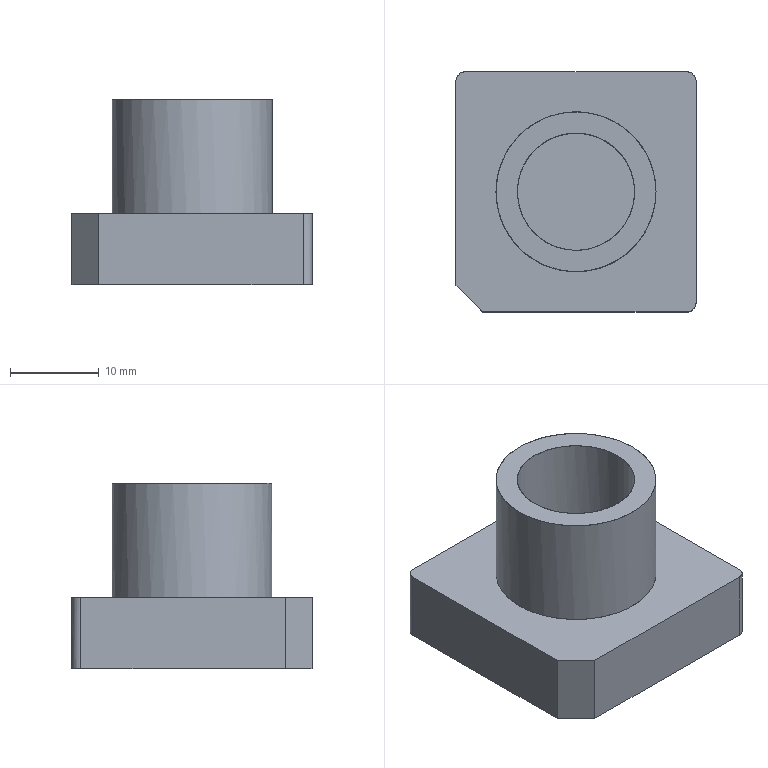NC program | PowerMill | posted with a generic post | part box 27 x 27 x 20.913 mm
Lines 1 to 1038 of 92133:
%
O0001
N104 ( POWERMILL CB  : 2026004.0)
N105 ( POST VER      : 2026.0.0.5161)
N106 ( OPTION FILE   : FANUC)
N107 ( OUTPUT WORKPLANE : WORLD)
N108 (  )
N109 ( TOOL LIST )
N110 (---------------------------------------)
N111 ( NO. | ID        | DIA.| TIP RAD|LENGTH)
N112 (---------------------------------------)
N113 (    1|D10C_1_1_1 |10.0 |  0.0   |76.36 )
N114 (    2|D4C_1_1    | 4.0 |  0.0   |68.12 )
N115 (    3|D10_1_1_1  |10.0 |  0.0   |76.08 )
N116 (   14|D4_1_1     | 4.0 |  0.0   |66.84 )
N117 (   13|TEXT_D4_1_1| 4.0 |  0.3   |68.16 )
N118 (---------------------------------------)
N119 (  )
N120 ( NUMBER OF TOOLPATHS: 11.0 )
N121 ( ESTIMATED PROGRAM DURATION: 0 HOURS 9 MIN 20 SEC)
N122 (  )
N123 G00 G21 G80 G40 G17
N124 G90
N125 G54
N126 G53 Z0.0
N127 (---------------)
N128 ( START TOOLPATH : 精公开粗01-扫面平行-D10C )
N129 (---------------)
N130 ( TOOL NO.    :1 )
N131 ( TOOL TYPE   : ENDMILL)
N132 ( TOOL ID     : D10C_1_1_1)
N133 ( TOOL DIA    : 10.0 LENGTH 76.36)
N134 T1
N135 M6
N136 S8000 M03
N137 G00 G90 X0.0 Y0.0
N138 G43 Z10.2 H1
N139
N140 G05 P10000 R4
N141 X21.28 Y16.28
N142 Z1.133
N143 G01 Z-0.067 F6000.0
N144 X16.28 F10000.0
N145 X-16.28
N146 Y10.8533
N147 X16.28
N148 Y5.4267
N149 X-16.28
N150 Y0.0
N151 X16.28
N152 Y-5.4267
N153 X-16.28
N154 Y-10.8533
N155 X16.28
N156 Y-16.28
N157 X-16.28
N158 X-21.28
N159 G00 Z10.2
N160 G05 P0
N161 (---------------)
N162 ( END TOOLPATH : 精公开粗01-扫面平行-D10C )
N163 (---------------)
N164 ( START TOOLPATH : 精公开粗01-外形偏置-D10C )
N165 (---------------)
N166 G00 X0.0 Y0.0 Z9.883
N167 G05 P10000 R4
N168 X22.054 Y5.4447
N169 Z0.6836
N170 G01 Z-0.5164 F6000.0
N171 X21.5265 F10000.0
N172 G03 X16.779 Y0.6972 I0.0 J-4.7475
N173 G01 Y-15.779
N174 G02 X15.779 Y-16.779 I-1.0 J0.0
N175 G01 X-15.779
N176 G02 X-16.779 Y-15.779 I0.0 J1.0
N177 G01 Y15.779
N178 G02 X-15.779 Y16.779 I1.0 J0.0
N179 G01 X15.779
N180 G02 X16.779 Y15.779 I0.0 J-1.0
N181 G01 Y0.6972
N182 X14.2597 Y0.5801
N183 X14.2687 Y0.3867
N184 Y-0.3867
N185 X14.2328 Y-1.1601
N186 X14.1427 Y-1.9336
N187 X14.0142 Y-2.707
N188 X13.8493 Y-3.4804
N189 X13.535 Y-4.5492
N190 X13.0486 Y-5.8007
N191 X12.7615 Y-6.4061
N192 X12.2358 Y-7.3476
N193 X11.7458 Y-8.121
N194 X11.1691 Y-8.8944
N195 X10.4413 Y-9.7288
N196 X9.7338 Y-10.4413
N197 X8.838 Y-11.2147
N198 X8.121 Y-11.7458
N199 X7.3476 Y-12.2446
N200 X6.5741 Y-12.6678
N201 X5.8007 Y-13.0486
N202 X4.5493 Y-13.535
N203 X3.4804 Y-13.8493
N204 X2.707 Y-14.02
N205 X1.9336 Y-14.1424
N206 X1.1601 Y-14.2328
N207 X-0.3867 Y-14.2747
N208 X-1.1601 Y-14.2328
N209 X-1.9336 Y-14.1478
N210 X-2.707 Y-14.0142
N211 X-3.4804 Y-13.8493
N212 X-4.5492 Y-13.535
N213 X-5.8007 Y-13.0486
N214 X-6.5741 Y-12.676
N215 X-7.3476 Y-12.2358
N216 X-8.121 Y-11.7458
N217 X-8.8944 Y-11.1654
N218 X-9.7288 Y-10.4413
N219 X-10.4413 Y-9.7404
N220 X-11.1654 Y-8.8944
N221 X-11.7458 Y-8.121
N222 X-11.9881 Y-7.7458
N223 X-12.6678 Y-6.5741
N224 X-13.0486 Y-5.8007
N225 X-13.535 Y-4.5492
N226 X-13.8493 Y-3.4804
N227 X-14.0164 Y-2.707
N228 X-14.1424 Y-1.9336
N229 X-14.2328 Y-1.1601
N230 X-14.2687 Y-0.3867
N231 Y0.3867
N232 X-14.2328 Y1.1601
N233 X-14.1424 Y1.9336
N234 X-14.0164 Y2.707
N235 X-13.8493 Y3.4804
N236 X-13.535 Y4.5493
N237 X-13.0486 Y5.8007
N238 X-12.6678 Y6.5741
N239 X-12.2358 Y7.3476
N240 X-11.7458 Y8.121
N241 X-11.1654 Y8.8944
N242 X-10.5096 Y9.6678
N243 X-9.7288 Y10.4413
N244 X-8.8944 Y11.1654
N245 X-8.121 Y11.7458
N246 X-7.7458 Y11.9881
N247 X-6.5741 Y12.676
N248 X-5.8007 Y13.0486
N249 X-4.5492 Y13.535
N250 X-3.4804 Y13.8493
N251 X-2.707 Y14.0142
N252 X-1.9336 Y14.1478
N253 X-1.1601 Y14.2328
N254 X-0.3867 Y14.2747
N255 X1.1601 Y14.2328
N256 X1.9336 Y14.1424
N257 X2.707 Y14.02
N258 X3.4804 Y13.8493
N259 X4.5493 Y13.535
N260 X5.8007 Y13.0486
N261 X6.5741 Y12.6678
N262 X7.3476 Y12.2446
N263 X8.121 Y11.7458
N264 X8.838 Y11.2147
N265 X9.7338 Y10.4413
N266 X10.4413 Y9.7288
N267 X11.1691 Y8.8944
N268 X11.7458 Y8.121
N269 X11.9881 Y7.7588
N270 X12.7615 Y6.4061
N271 X13.0486 Y5.8007
N272 X13.535 Y4.5493
N273 X13.8493 Y3.4804
N274 X14.0142 Y2.707
N275 X14.1427 Y1.9336
N276 X14.2328 Y1.1601
N277 X14.2597 Y0.5801
N278 X16.779 Y0.6972
N279 G00 Z3.2842
N280 G01 X22.054 Y5.4447
N281 G00 Z0.2842
N282 G01 Z-0.9158 F6000.0
N283 X21.5265 F10000.0
N284 G03 X16.779 Y0.6972 I0.0 J-4.7475
N285 G01 Y-15.779
N286 G02 X15.779 Y-16.779 I-1.0 J0.0
N287 G01 X-15.779
N288 G02 X-16.779 Y-15.779 I0.0 J1.0
N289 G01 Y15.779
N290 G02 X-15.779 Y16.779 I1.0 J0.0
N291 G01 X15.779
N292 G02 X16.779 Y15.779 I0.0 J-1.0
N293 G01 Y0.6972
N294 X14.2597 Y0.5801
N295 X14.2687 Y0.3867
N296 Y-0.3867
N297 X14.2328 Y-1.1601
N298 X14.1427 Y-1.9336
N299 X14.0142 Y-2.707
N300 X13.8493 Y-3.4804
N301 X13.535 Y-4.5492
N302 X13.0486 Y-5.8007
N303 X12.7615 Y-6.4061
N304 X12.2358 Y-7.3476
N305 X11.7458 Y-8.121
N306 X11.1691 Y-8.8944
N307 X10.4413 Y-9.7288
N308 X9.7338 Y-10.4413
N309 X8.838 Y-11.2147
N310 X8.121 Y-11.7458
N311 X7.3476 Y-12.2446
N312 X6.5741 Y-12.6678
N313 X5.8007 Y-13.0486
N314 X4.5493 Y-13.535
N315 X3.4804 Y-13.8493
N316 X2.707 Y-14.02
N317 X1.9336 Y-14.1424
N318 X1.1601 Y-14.2328
N319 X-0.3867 Y-14.2747
N320 X-1.1601 Y-14.2328
N321 X-1.9336 Y-14.1478
N322 X-2.707 Y-14.0142
N323 X-3.4804 Y-13.8493
N324 X-4.5492 Y-13.535
N325 X-5.8007 Y-13.0486
N326 X-6.5741 Y-12.676
N327 X-7.3476 Y-12.2358
N328 X-8.121 Y-11.7458
N329 X-8.8944 Y-11.1654
N330 X-9.7288 Y-10.4413
N331 X-10.4413 Y-9.7404
N332 X-11.1654 Y-8.8944
N333 X-11.7458 Y-8.121
N334 X-11.9881 Y-7.7459
N335 X-12.6678 Y-6.5741
N336 X-13.0486 Y-5.8007
N337 X-13.535 Y-4.5492
N338 X-13.8493 Y-3.4804
N339 X-14.0164 Y-2.707
N340 X-14.1424 Y-1.9336
N341 X-14.2328 Y-1.1601
N342 X-14.2687 Y-0.3867
N343 Y0.3867
N344 X-14.2328 Y1.1601
N345 X-14.1424 Y1.9336
N346 X-14.0164 Y2.707
N347 X-13.8493 Y3.4804
N348 X-13.535 Y4.5493
N349 X-13.0486 Y5.8007
N350 X-12.6678 Y6.5741
N351 X-12.2358 Y7.3476
N352 X-11.7458 Y8.121
N353 X-11.1654 Y8.8944
N354 X-10.5096 Y9.6678
N355 X-9.7288 Y10.4413
N356 X-8.8944 Y11.1654
N357 X-8.121 Y11.7458
N358 X-7.7459 Y11.9881
N359 X-6.5741 Y12.676
N360 X-5.8007 Y13.0486
N361 X-4.5492 Y13.535
N362 X-3.4804 Y13.8493
N363 X-2.707 Y14.0142
N364 X-1.9336 Y14.1478
N365 X-1.1601 Y14.2328
N366 X-0.3867 Y14.2747
N367 X1.1601 Y14.2328
N368 X1.9336 Y14.1424
N369 X2.707 Y14.02
N370 X3.4804 Y13.8493
N371 X4.5493 Y13.535
N372 X5.8007 Y13.0486
N373 X6.5741 Y12.6678
N374 X7.3476 Y12.2446
N375 X8.121 Y11.7458
N376 X8.838 Y11.2147
N377 X9.7338 Y10.4413
N378 X10.4413 Y9.7288
N379 X11.1691 Y8.8944
N380 X11.7458 Y8.121
N381 X11.9881 Y7.7588
N382 X12.7615 Y6.4061
N383 X13.0486 Y5.8007
N384 X13.535 Y4.5493
N385 X13.8493 Y3.4804
N386 X14.0142 Y2.707
N387 X14.1427 Y1.9336
N388 X14.2328 Y1.1601
N389 X14.2597 Y0.5801
N390 X16.779 Y0.6972
N391 G00 Z2.8848
N392 G01 X22.054 Y5.4447
N393 G00 Z-0.1152
N394 G01 Z-1.3152 F6000.0
N395 X21.5265 F10000.0
N396 G03 X16.779 Y0.6972 I0.0 J-4.7475
N397 G01 Y-15.779
N398 G02 X15.779 Y-16.779 I-1.0 J0.0
N399 G01 X-15.779
N400 G02 X-16.779 Y-15.779 I0.0 J1.0
N401 G01 Y15.779
N402 G02 X-15.779 Y16.779 I1.0 J0.0
N403 G01 X15.779
N404 G02 X16.779 Y15.779 I0.0 J-1.0
N405 G01 Y0.6972
N406 X14.2597 Y0.5801
N407 X14.2687 Y0.3867
N408 Y-0.3867
N409 X14.2328 Y-1.1601
N410 X14.1427 Y-1.9336
N411 X14.0142 Y-2.707
N412 X13.8493 Y-3.4804
N413 X13.535 Y-4.5492
N414 X13.0486 Y-5.8007
N415 X12.7615 Y-6.4061
N416 X12.2358 Y-7.3476
N417 X11.7458 Y-8.121
N418 X11.1691 Y-8.8944
N419 X10.4413 Y-9.7288
N420 X9.7338 Y-10.4413
N421 X8.838 Y-11.2147
N422 X8.121 Y-11.7458
N423 X7.3476 Y-12.2446
N424 X6.5741 Y-12.6678
N425 X5.8007 Y-13.0486
N426 X4.5493 Y-13.535
N427 X3.4804 Y-13.8493
N428 X2.707 Y-14.02
N429 X1.9336 Y-14.1424
N430 X1.1601 Y-14.2328
N431 X-0.3867 Y-14.2747
N432 X-1.1601 Y-14.2328
N433 X-1.9336 Y-14.1478
N434 X-2.707 Y-14.0142
N435 X-3.4804 Y-13.8493
N436 X-4.5492 Y-13.535
N437 X-5.8007 Y-13.0486
N438 X-6.5741 Y-12.676
N439 X-7.3476 Y-12.2358
N440 X-8.121 Y-11.7458
N441 X-8.8944 Y-11.1654
N442 X-9.7288 Y-10.4413
N443 X-10.4413 Y-9.7404
N444 X-11.1654 Y-8.8944
N445 X-11.7458 Y-8.121
N446 X-11.9881 Y-7.7459
N447 X-12.6678 Y-6.5741
N448 X-13.0486 Y-5.8007
N449 X-13.535 Y-4.5492
N450 X-13.8493 Y-3.4804
N451 X-14.0164 Y-2.707
N452 X-14.1424 Y-1.9336
N453 X-14.2328 Y-1.1601
N454 X-14.2687 Y-0.3867
N455 Y0.3867
N456 X-14.2328 Y1.1601
N457 X-14.1424 Y1.9336
N458 X-14.0164 Y2.707
N459 X-13.8493 Y3.4804
N460 X-13.535 Y4.5493
N461 X-13.0486 Y5.8007
N462 X-12.6678 Y6.5741
N463 X-12.2358 Y7.3476
N464 X-11.7458 Y8.121
N465 X-11.1654 Y8.8944
N466 X-10.5096 Y9.6678
N467 X-9.7288 Y10.4413
N468 X-8.8944 Y11.1654
N469 X-8.121 Y11.7458
N470 X-7.7459 Y11.9881
N471 X-6.5741 Y12.676
N472 X-5.8007 Y13.0486
N473 X-4.5492 Y13.535
N474 X-3.4804 Y13.8493
N475 X-2.707 Y14.0142
N476 X-1.9336 Y14.1478
N477 X-1.1601 Y14.2328
N478 X-0.3867 Y14.2747
N479 X1.1601 Y14.2328
N480 X1.9336 Y14.1424
N481 X2.707 Y14.02
N482 X3.4804 Y13.8493
N483 X4.5493 Y13.535
N484 X5.8007 Y13.0486
N485 X6.5741 Y12.6678
N486 X7.3476 Y12.2446
N487 X8.121 Y11.7458
N488 X8.838 Y11.2147
N489 X9.7338 Y10.4413
N490 X10.4413 Y9.7288
N491 X11.1691 Y8.8944
N492 X11.7458 Y8.121
N493 X11.9881 Y7.7588
N494 X12.7615 Y6.4061
N495 X13.0486 Y5.8007
N496 X13.535 Y4.5493
N497 X13.8493 Y3.4804
N498 X14.0142 Y2.707
N499 X14.1427 Y1.9336
N500 X14.2328 Y1.1601
N501 X14.2597 Y0.5801
N502 X16.779 Y0.6972
N503 G00 Z2.4854
N504 G01 X22.054 Y5.4447
N505 G00 Z-0.5146
N506 G01 Z-1.7146 F6000.0
N507 X21.5265 F10000.0
N508 G03 X16.779 Y0.6972 I0.0 J-4.7475
N509 G01 Y-15.779
N510 G02 X15.779 Y-16.779 I-1.0 J0.0
N511 G01 X-15.779
N512 G02 X-16.779 Y-15.779 I0.0 J1.0
N513 G01 Y15.779
N514 G02 X-15.779 Y16.779 I1.0 J0.0
N515 G01 X15.779
N516 G02 X16.779 Y15.779 I0.0 J-1.0
N517 G01 Y0.6972
N518 X14.2597 Y0.5801
N519 X14.2687 Y0.3867
N520 Y-0.3867
N521 X14.2328 Y-1.1601
N522 X14.1427 Y-1.9336
N523 X14.0142 Y-2.707
N524 X13.8493 Y-3.4804
N525 X13.535 Y-4.5492
N526 X13.0486 Y-5.8007
N527 X12.7615 Y-6.4061
N528 X12.2358 Y-7.3476
N529 X11.7458 Y-8.121
N530 X11.1691 Y-8.8944
N531 X10.4413 Y-9.7288
N532 X9.7338 Y-10.4413
N533 X8.838 Y-11.2147
N534 X8.121 Y-11.7458
N535 X7.3476 Y-12.2446
N536 X6.5741 Y-12.6678
N537 X5.8007 Y-13.0486
N538 X4.5493 Y-13.535
N539 X3.4804 Y-13.8493
N540 X2.707 Y-14.02
N541 X1.9336 Y-14.1424
N542 X1.1601 Y-14.2328
N543 X-0.3867 Y-14.2747
N544 X-1.1601 Y-14.2328
N545 X-1.9336 Y-14.1478
N546 X-2.707 Y-14.0142
N547 X-3.4804 Y-13.8493
N548 X-4.5492 Y-13.535
N549 X-5.8007 Y-13.0486
N550 X-6.5741 Y-12.676
N551 X-7.3476 Y-12.2358
N552 X-8.121 Y-11.7458
N553 X-8.8944 Y-11.1654
N554 X-9.7288 Y-10.4413
N555 X-10.4413 Y-9.7404
N556 X-11.1654 Y-8.8944
N557 X-11.7458 Y-8.121
N558 X-11.9881 Y-7.7459
N559 X-12.6678 Y-6.5741
N560 X-13.0486 Y-5.8007
N561 X-13.535 Y-4.5492
N562 X-13.8493 Y-3.4804
N563 X-14.0164 Y-2.707
N564 X-14.1424 Y-1.9336
N565 X-14.2328 Y-1.1601
N566 X-14.2687 Y-0.3867
N567 Y0.3867
N568 X-14.2328 Y1.1601
N569 X-14.1424 Y1.9336
N570 X-14.0164 Y2.707
N571 X-13.8493 Y3.4804
N572 X-13.535 Y4.5493
N573 X-13.0486 Y5.8007
N574 X-12.6678 Y6.5741
N575 X-12.2358 Y7.3476
N576 X-11.7458 Y8.121
N577 X-11.1654 Y8.8944
N578 X-10.5096 Y9.6678
N579 X-9.7288 Y10.4413
N580 X-8.8944 Y11.1654
N581 X-8.121 Y11.7458
N582 X-7.7459 Y11.9881
N583 X-6.5741 Y12.676
N584 X-5.8007 Y13.0486
N585 X-4.5492 Y13.535
N586 X-3.4804 Y13.8493
N587 X-2.707 Y14.0142
N588 X-1.9336 Y14.1478
N589 X-1.1601 Y14.2328
N590 X-0.3867 Y14.2747
N591 X1.1601 Y14.2328
N592 X1.9336 Y14.1424
N593 X2.707 Y14.02
N594 X3.4804 Y13.8493
N595 X4.5493 Y13.535
N596 X5.8007 Y13.0486
N597 X6.5741 Y12.6678
N598 X7.3476 Y12.2446
N599 X8.121 Y11.7458
N600 X8.838 Y11.2147
N601 X9.7338 Y10.4413
N602 X10.4413 Y9.7288
N603 X11.1691 Y8.8944
N604 X11.7458 Y8.121
N605 X11.9881 Y7.7588
N606 X12.7615 Y6.4061
N607 X13.0486 Y5.8007
N608 X13.535 Y4.5493
N609 X13.8493 Y3.4804
N610 X14.0142 Y2.707
N611 X14.1427 Y1.9336
N612 X14.2328 Y1.1601
N613 X14.2597 Y0.5801
N614 X16.779 Y0.6972
N615 G00 Z2.086
N616 G01 X22.054 Y5.4447
N617 G00 Z-0.914
N618 G01 Z-2.114 F6000.0
N619 X21.5265 F10000.0
N620 G03 X16.779 Y0.6972 I0.0 J-4.7475
N621 G01 Y-15.779
N622 G02 X15.779 Y-16.779 I-1.0 J0.0
N623 G01 X-15.779
N624 G02 X-16.779 Y-15.779 I0.0 J1.0
N625 G01 Y15.779
N626 G02 X-15.779 Y16.779 I1.0 J0.0
N627 G01 X15.779
N628 G02 X16.779 Y15.779 I0.0 J-1.0
N629 G01 Y0.6972
N630 X14.2597 Y0.5801
N631 X14.2687 Y0.3867
N632 Y-0.3867
N633 X14.2328 Y-1.1601
N634 X14.1427 Y-1.9336
N635 X14.0142 Y-2.707
N636 X13.8493 Y-3.4804
N637 X13.535 Y-4.5492
N638 X13.0486 Y-5.8007
N639 X12.7615 Y-6.4061
N640 X12.2358 Y-7.3476
N641 X11.7458 Y-8.121
N642 X11.1691 Y-8.8944
N643 X10.4413 Y-9.7288
N644 X9.7338 Y-10.4413
N645 X8.838 Y-11.2147
N646 X8.121 Y-11.7458
N647 X7.3476 Y-12.2446
N648 X6.5741 Y-12.6678
N649 X5.8007 Y-13.0486
N650 X4.5493 Y-13.535
N651 X3.4804 Y-13.8493
N652 X2.707 Y-14.02
N653 X1.9336 Y-14.1424
N654 X1.1601 Y-14.2328
N655 X-0.3867 Y-14.2747
N656 X-1.1601 Y-14.2328
N657 X-1.9336 Y-14.1478
N658 X-2.707 Y-14.0142
N659 X-3.4804 Y-13.8493
N660 X-4.5492 Y-13.535
N661 X-5.8007 Y-13.0486
N662 X-6.5741 Y-12.676
N663 X-7.3476 Y-12.2358
N664 X-8.121 Y-11.7458
N665 X-8.8944 Y-11.1654
N666 X-9.7288 Y-10.4413
N667 X-10.4413 Y-9.7404
N668 X-11.1654 Y-8.8944
N669 X-11.7458 Y-8.121
N670 X-11.9881 Y-7.7459
N671 X-12.6678 Y-6.5741
N672 X-13.0486 Y-5.8007
N673 X-13.535 Y-4.5492
N674 X-13.8493 Y-3.4804
N675 X-14.0164 Y-2.707
N676 X-14.1424 Y-1.9336
N677 X-14.2328 Y-1.1601
N678 X-14.2687 Y-0.3867
N679 Y0.3867
N680 X-14.2328 Y1.1601
N681 X-14.1424 Y1.9336
N682 X-14.0164 Y2.707
N683 X-13.8493 Y3.4804
N684 X-13.535 Y4.5493
N685 X-13.0486 Y5.8007
N686 X-12.6678 Y6.5741
N687 X-12.2358 Y7.3476
N688 X-11.7458 Y8.121
N689 X-11.1654 Y8.8944
N690 X-10.5096 Y9.6678
N691 X-9.7288 Y10.4413
N692 X-8.8944 Y11.1654
N693 X-8.121 Y11.7458
N694 X-7.7459 Y11.9881
N695 X-6.5741 Y12.676
N696 X-5.8007 Y13.0486
N697 X-4.5492 Y13.535
N698 X-3.4804 Y13.8493
N699 X-2.707 Y14.0142
N700 X-1.9336 Y14.1478
N701 X-1.1601 Y14.2328
N702 X-0.3867 Y14.2747
N703 X1.1601 Y14.2328
N704 X1.9336 Y14.1424
N705 X2.707 Y14.02
N706 X3.4804 Y13.8493
N707 X4.5493 Y13.535
N708 X5.8007 Y13.0486
N709 X6.5741 Y12.6678
N710 X7.3476 Y12.2446
N711 X8.121 Y11.7458
N712 X8.838 Y11.2147
N713 X9.7338 Y10.4413
N714 X10.4413 Y9.7288
N715 X11.1691 Y8.8944
N716 X11.7458 Y8.121
N717 X11.9881 Y7.7588
N718 X12.7615 Y6.4061
N719 X13.0486 Y5.8007
N720 X13.535 Y4.5493
N721 X13.8493 Y3.4804
N722 X14.0142 Y2.707
N723 X14.1427 Y1.9336
N724 X14.2328 Y1.1601
N725 X14.2597 Y0.5801
N726 X16.779 Y0.6972
N727 G00 Z1.6867
N728 G01 X22.054 Y5.4447
N729 G00 Z-1.3133
N730 G01 Z-2.5134 F6000.0
N731 X21.5265 F10000.0
N732 G03 X16.779 Y0.6972 I0.0 J-4.7475
N733 G01 Y-15.779
N734 G02 X15.779 Y-16.779 I-1.0 J0.0
N735 G01 X-15.779
N736 G02 X-16.779 Y-15.779 I0.0 J1.0
N737 G01 Y15.779
N738 G02 X-15.779 Y16.779 I1.0 J0.0
N739 G01 X15.779
N740 G02 X16.779 Y15.779 I0.0 J-1.0
N741 G01 Y0.6972
N742 X14.2597 Y0.5801
N743 X14.2687 Y0.3867
N744 Y-0.3867
N745 X14.2328 Y-1.1601
N746 X14.1427 Y-1.9336
N747 X14.0142 Y-2.707
N748 X13.8493 Y-3.4804
N749 X13.535 Y-4.5492
N750 X13.0486 Y-5.8007
N751 X12.7615 Y-6.4061
N752 X12.2358 Y-7.3476
N753 X11.7458 Y-8.121
N754 X11.1691 Y-8.8944
N755 X10.4413 Y-9.7288
N756 X9.7338 Y-10.4413
N757 X8.838 Y-11.2147
N758 X8.121 Y-11.7458
N759 X7.3476 Y-12.2446
N760 X6.5741 Y-12.6678
N761 X5.8007 Y-13.0486
N762 X4.5493 Y-13.535
N763 X3.4804 Y-13.8493
N764 X2.707 Y-14.02
N765 X1.9336 Y-14.1424
N766 X1.1601 Y-14.2328
N767 X-0.3867 Y-14.2747
N768 X-1.1601 Y-14.2328
N769 X-1.9336 Y-14.1478
N770 X-2.707 Y-14.0142
N771 X-3.4804 Y-13.8493
N772 X-4.5492 Y-13.535
N773 X-5.8007 Y-13.0486
N774 X-6.5741 Y-12.676
N775 X-7.3476 Y-12.2358
N776 X-8.121 Y-11.7458
N777 X-8.8944 Y-11.1654
N778 X-9.7288 Y-10.4413
N779 X-10.4413 Y-9.7404
N780 X-11.1654 Y-8.8944
N781 X-11.7458 Y-8.121
N782 X-11.9881 Y-7.7459
N783 X-12.6678 Y-6.5741
N784 X-13.0486 Y-5.8007
N785 X-13.535 Y-4.5492
N786 X-13.8493 Y-3.4804
N787 X-14.0164 Y-2.707
N788 X-14.1424 Y-1.9336
N789 X-14.2328 Y-1.1601
N790 X-14.2687 Y-0.3867
N791 Y0.3867
N792 X-14.2328 Y1.1601
N793 X-14.1424 Y1.9336
N794 X-14.0164 Y2.707
N795 X-13.8493 Y3.4804
N796 X-13.535 Y4.5493
N797 X-13.0486 Y5.8007
N798 X-12.6678 Y6.5741
N799 X-12.2358 Y7.3476
N800 X-11.7458 Y8.121
N801 X-11.1654 Y8.8944
N802 X-10.5096 Y9.6678
N803 X-9.7288 Y10.4413
N804 X-8.8944 Y11.1654
N805 X-8.121 Y11.7458
N806 X-7.7459 Y11.9881
N807 X-6.5741 Y12.676
N808 X-5.8007 Y13.0486
N809 X-4.5492 Y13.535
N810 X-3.4804 Y13.8493
N811 X-2.707 Y14.0142
N812 X-1.9336 Y14.1478
N813 X-1.1601 Y14.2328
N814 X-0.3867 Y14.2747
N815 X1.1601 Y14.2328
N816 X1.9336 Y14.1424
N817 X2.707 Y14.02
N818 X3.4804 Y13.8493
N819 X4.5493 Y13.535
N820 X5.8007 Y13.0486
N821 X6.5741 Y12.6678
N822 X7.3476 Y12.2446
N823 X8.121 Y11.7458
N824 X8.838 Y11.2147
N825 X9.7338 Y10.4413
N826 X10.4413 Y9.7288
N827 X11.1691 Y8.8944
N828 X11.7458 Y8.121
N829 X11.9881 Y7.7588
N830 X12.7615 Y6.4061
N831 X13.0486 Y5.8007
N832 X13.535 Y4.5493
N833 X13.8493 Y3.4804
N834 X14.0142 Y2.707
N835 X14.1427 Y1.9336
N836 X14.2328 Y1.1601
N837 X14.2597 Y0.5801
N838 X16.779 Y0.6972
N839 G00 Z1.2873
N840 G01 X22.054 Y5.4447
N841 G00 Z-1.7127
N842 G01 Z-2.9127 F6000.0
N843 X21.5265 F10000.0
N844 G03 X16.779 Y0.6972 I0.0 J-4.7475
N845 G01 Y-15.779
N846 G02 X15.779 Y-16.779 I-1.0 J0.0
N847 G01 X-15.779
N848 G02 X-16.779 Y-15.779 I0.0 J1.0
N849 G01 Y15.779
N850 G02 X-15.779 Y16.779 I1.0 J0.0
N851 G01 X15.779
N852 G02 X16.779 Y15.779 I0.0 J-1.0
N853 G01 Y0.6972
N854 X14.2597 Y0.5801
N855 X14.2687 Y0.3867
N856 Y-0.3867
N857 X14.2328 Y-1.1601
N858 X14.1427 Y-1.9336
N859 X14.0142 Y-2.707
N860 X13.8493 Y-3.4804
N861 X13.535 Y-4.5493
N862 X13.0486 Y-5.8007
N863 X12.7615 Y-6.4061
N864 X12.2359 Y-7.3476
N865 X11.7458 Y-8.121
N866 X11.1691 Y-8.8944
N867 X10.4413 Y-9.7288
N868 X9.7338 Y-10.4413
N869 X8.838 Y-11.2147
N870 X8.121 Y-11.7458
N871 X7.3476 Y-12.2446
N872 X6.5741 Y-12.6678
N873 X5.8007 Y-13.0486
N874 X4.5493 Y-13.535
N875 X3.4804 Y-13.8493
N876 X2.707 Y-14.02
N877 X1.9336 Y-14.1424
N878 X1.1601 Y-14.2328
N879 X-0.3867 Y-14.2747
N880 X-1.1601 Y-14.2328
N881 X-1.9336 Y-14.1478
N882 X-2.707 Y-14.0142
N883 X-3.4804 Y-13.8493
N884 X-4.5493 Y-13.535
N885 X-5.8007 Y-13.0486
N886 X-6.5741 Y-12.676
N887 X-7.3476 Y-12.2359
N888 X-8.121 Y-11.7458
N889 X-8.8944 Y-11.1654
N890 X-9.7288 Y-10.4413
N891 X-10.4413 Y-9.7404
N892 X-11.1654 Y-8.8944
N893 X-11.7458 Y-8.121
N894 X-11.9881 Y-7.7459
N895 X-12.6678 Y-6.5741
N896 X-13.0486 Y-5.8007
N897 X-13.535 Y-4.5493
N898 X-13.8493 Y-3.4804
N899 X-14.0164 Y-2.707
N900 X-14.1424 Y-1.9336
N901 X-14.2328 Y-1.1601
N902 X-14.2687 Y-0.3867
N903 Y0.3867
N904 X-14.2328 Y1.1601
N905 X-14.1424 Y1.9336
N906 X-14.0164 Y2.707
N907 X-13.8493 Y3.4804
N908 X-13.535 Y4.5493
N909 X-13.0486 Y5.8007
N910 X-12.6678 Y6.5741
N911 X-12.2359 Y7.3476
N912 X-11.7458 Y8.121
N913 X-11.1654 Y8.8944
N914 X-10.5096 Y9.6678
N915 X-9.7288 Y10.4413
N916 X-8.8944 Y11.1654
N917 X-8.121 Y11.7458
N918 X-7.7459 Y11.9881
N919 X-6.5741 Y12.676
N920 X-5.8007 Y13.0486
N921 X-4.5493 Y13.535
N922 X-3.4804 Y13.8493
N923 X-2.707 Y14.0142
N924 X-1.9336 Y14.1478
N925 X-1.1601 Y14.2328
N926 X-0.3867 Y14.2747
N927 X1.1601 Y14.2328
N928 X1.9336 Y14.1424
N929 X2.707 Y14.02
N930 X3.4804 Y13.8493
N931 X4.5493 Y13.535
N932 X5.8007 Y13.0486
N933 X6.5741 Y12.6678
N934 X7.3476 Y12.2446
N935 X8.121 Y11.7458
N936 X8.838 Y11.2147
N937 X9.7338 Y10.4413
N938 X10.4413 Y9.7288
N939 X11.1691 Y8.8944
N940 X11.7458 Y8.121
N941 X11.9881 Y7.7588
N942 X12.7615 Y6.4061
N943 X13.0486 Y5.8007
N944 X13.535 Y4.5493
N945 X13.8493 Y3.4804
N946 X14.0142 Y2.707
N947 X14.1427 Y1.9336
N948 X14.2328 Y1.1601
N949 X14.2597 Y0.5801
N950 X16.779 Y0.6972
N951 G00 Z0.8879
N952 G01 X22.054 Y5.4447
N953 G00 Z-2.1121
N954 G01 Z-3.3121 F6000.0
N955 X21.5265 F10000.0
N956 G03 X16.779 Y0.6972 I0.0 J-4.7475
N957 G01 Y-15.779
N958 G02 X15.779 Y-16.779 I-1.0 J0.0
N959 G01 X-15.779
N960 G02 X-16.779 Y-15.779 I0.0 J1.0
N961 G01 Y15.779
N962 G02 X-15.779 Y16.779 I1.0 J0.0
N963 G01 X15.779
N964 G02 X16.779 Y15.779 I0.0 J-1.0
N965 G01 Y0.6972
N966 X14.2597 Y0.5801
N967 X14.2687 Y0.3867
N968 Y-0.3867
N969 X14.2328 Y-1.1601
N970 X14.1427 Y-1.9336
N971 X14.0142 Y-2.707
N972 X13.8493 Y-3.4804
N973 X13.535 Y-4.5493
N974 X13.0486 Y-5.8007
N975 X12.7615 Y-6.4061
N976 X12.2359 Y-7.3476
N977 X11.7458 Y-8.121
N978 X11.1691 Y-8.8944
N979 X10.4413 Y-9.7288
N980 X9.7339 Y-10.4413
N981 X8.838 Y-11.2147
N982 X8.121 Y-11.7458
N983 X7.3476 Y-12.2446
N984 X6.5741 Y-12.6678
N985 X5.8007 Y-13.0486
N986 X4.5493 Y-13.535
N987 X3.4804 Y-13.8493
N988 X2.707 Y-14.02
N989 X1.9336 Y-14.1424
N990 X1.1601 Y-14.2328
N991 X-0.3867 Y-14.2747
N992 X-1.1601 Y-14.2328
N993 X-1.9336 Y-14.1479
N994 X-2.707 Y-14.0142
N995 X-3.4804 Y-13.8493
N996 X-4.5493 Y-13.535
N997 X-5.8007 Y-13.0486
N998 X-6.5741 Y-12.676
N999 X-7.3476 Y-12.2359
N1000 X-8.121 Y-11.7458
N1001 X-8.8944 Y-11.1654
N1002 X-9.7288 Y-10.4413
N1003 X-10.4413 Y-9.7404
N1004 X-11.1654 Y-8.8944
N1005 X-11.7458 Y-8.121
N1006 X-11.9881 Y-7.7459
N1007 X-12.6678 Y-6.5741
N1008 X-13.0486 Y-5.8007
N1009 X-13.535 Y-4.5493
N1010 X-13.8493 Y-3.4804
N1011 X-14.0164 Y-2.707
N1012 X-14.1424 Y-1.9336
N1013 X-14.2328 Y-1.1601
N1014 X-14.2687 Y-0.3867
N1015 Y0.3867
N1016 X-14.2328 Y1.1601
N1017 X-14.1424 Y1.9336
N1018 X-14.0164 Y2.707
N1019 X-13.8493 Y3.4804
N1020 X-13.535 Y4.5493
N1021 X-13.0486 Y5.8007
N1022 X-12.6678 Y6.5741
N1023 X-12.2359 Y7.3476
N1024 X-11.7458 Y8.121
N1025 X-11.1654 Y8.8944
N1026 X-10.5096 Y9.6678
N1027 X-9.7288 Y10.4413
N1028 X-8.8944 Y11.1654
N1029 X-8.121 Y11.7458
N1030 X-7.7459 Y11.9881
N1031 X-6.5741 Y12.676
N1032 X-5.8007 Y13.0486
N1033 X-4.5493 Y13.535
N1034 X-3.4804 Y13.8493
N1035 X-2.707 Y14.0142
N1036 X-1.9336 Y14.1479
N1037 X-1.1601 Y14.2328
N1038 X-0.3867 Y14.2747
N1039 X1.1601 Y14.2328
N1040 X1.9336 Y14.1424
N1041 X2.707 Y14.02
N1042 X3.4804 Y13.8493
N1043 X4.5493 Y13.535
N1044 X5.8007 Y13.0486
N1045 X6.5741 Y12.6678
N1046 X7.3476 Y12.2446
N1047 X8.121 Y11.7458
N1048 X8.838 Y11.2147
N1049 X9.7339 Y10.4413
N1050 X10.4413 Y9.7288
N1051 X11.1691 Y8.8944
N1052 X11.7458 Y8.121
N1053 X11.9881 Y7.7588
N1054 X12.7615 Y6.4061
N1055 X13.0486 Y5.8007
N1056 X13.535 Y4.5493
N1057 X13.8493 Y3.4804
N1058 X14.0142 Y2.707
N1059 X14.1427 Y1.9336
N1060 X14.2328 Y1.1601
N1061 X14.2597 Y0.5801
N1062 X16.779 Y0.6972
N1063 G00 Z0.4885
N1064 G01 X22.054 Y5.4447
N1065 G00 Z-2.5115
N1066 G01 Z-3.7115 F6000.0
N1067 X21.5265 F10000.0
N1068 G03 X16.779 Y0.6972 I0.0 J-4.7475
N1069 G01 Y-15.779
N1070 G02 X15.779 Y-16.779 I-1.0 J0.0
N1071 G01 X-15.779
N1072 G02 X-16.779 Y-15.779 I0.0 J1.0
N1073 G01 Y15.779
N1074 G02 X-15.779 Y16.779 I1.0 J0.0
N1075 G01 X15.779
N1076 G02 X16.779 Y15.779 I0.0 J-1.0
N1077 G01 Y0.6972
N1078 X14.2597 Y0.5801
N1079 X14.2687 Y0.3867
N1080 Y-0.3867
N1081 X14.2328 Y-1.1601
N1082 X14.1427 Y-1.9336
N1083 X14.0142 Y-2.707
N1084 X13.8493 Y-3.4804
N1085 X13.535 Y-4.5493
N1086 X13.0486 Y-5.8007
N1087 X12.7615 Y-6.4061
N1088 X12.2359 Y-7.3476
N1089 X11.7458 Y-8.121
N1090 X11.1691 Y-8.8944
N1091 X10.4413 Y-9.7288
N1092 X9.7339 Y-10.4413
N1093 X8.838 Y-11.2147
N1094 X8.121 Y-11.7458
N1095 X7.3476 Y-12.2446
N1096 X6.5741 Y-12.6678
N1097 X5.8007 Y-13.0486
N1098 X4.5493 Y-13.535
N1099 X3.4804 Y-13.8493
N1100 X2.707 Y-14.02
N1101 X1.9336 Y-14.1424
N1102 X1.1601 Y-14.2328
N1103 X-0.3867 Y-14.2747
N1104 X-1.1601 Y-14.2328
N1105 X-1.9336 Y-14.1479
N1106 X-2.707 Y-14.0142
N1107 X-3.4804 Y-13.8493
N1108 X-4.5493 Y-13.535
N1109 X-5.8007 Y-13.0486
N1110 X-6.5741 Y-12.676
N1111 X-7.3476 Y-12.2359
N1112 X-8.121 Y-11.7458
N1113 X-8.8944 Y-11.1654
N1114 X-9.7288 Y-10.4413
N1115 X-10.4413 Y-9.7404
N1116 X-11.1654 Y-8.8944
N1117 X-11.7458 Y-8.121
N1118 X-11.9881 Y-7.7459
N1119 X-12.6678 Y-6.5741
N1120 X-13.0486 Y-5.8007
N1121 X-13.535 Y-4.5493
N1122 X-13.8493 Y-3.4804
N1123 X-14.0164 Y-2.707
N1124 X-14.1424 Y-1.9336
N1125 X-14.2328 Y-1.1601
N1126 X-14.2687 Y-0.3867
N1127 Y0.3867
N1128 X-14.2328 Y1.1601
N1129 X-14.1424 Y1.9336
N1130 X-14.0164 Y2.707
N1131 X-13.8493 Y3.4804
N1132 X-13.535 Y4.5493
N1133 X-13.0486 Y5.8007
N1134 X-12.6678 Y6.5741
N1135 X-12.2359 Y7.3476